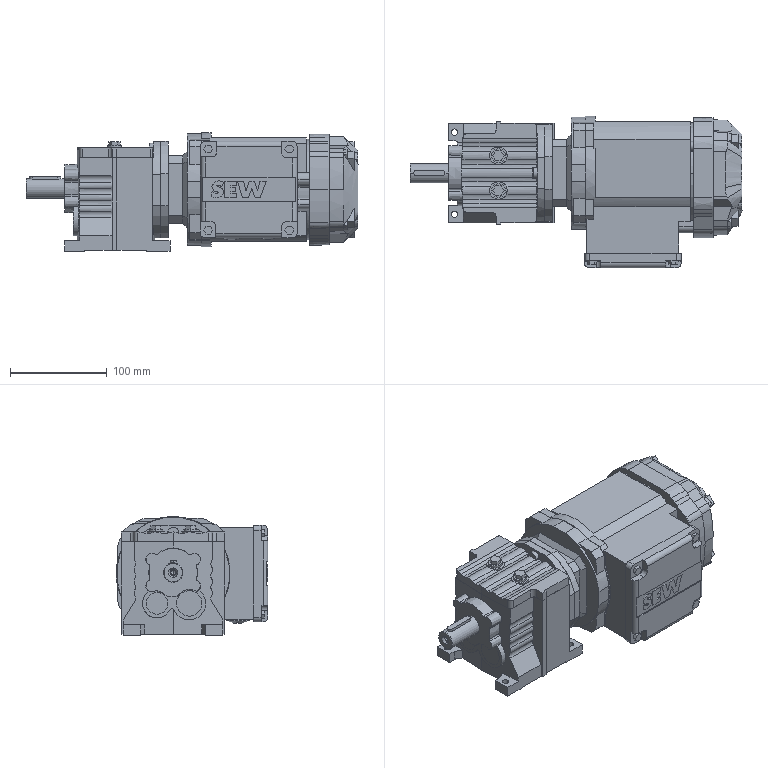Part | STEP file | 12 solids | 626 faces | box 343.5 x 157 x 122.87 mm | volume 3393544 mm3 | plane 349 | cylinder 187 | cone 58 | spline 32 | commonest cylinder face diameters 0.1 x31 22 x19 10 x16 12 x14 6.6 x8 7.219 x8